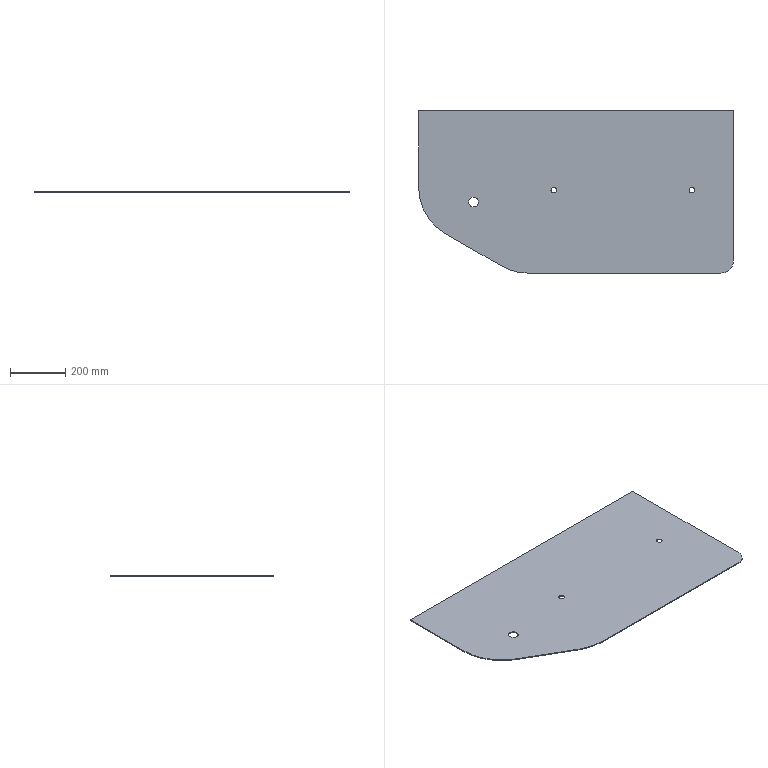Part | SolidWorks | features Extrusion 1 | 1 solid | 16 faces | box 1139 x 587 x 3 mm | volume 1890389 mm3 | cylinder 9 | plane 7 | commonest cylinder face diameters 20 x4 35 x2 390 x2 90 x1
STEP:
#1=CARTESIAN_POINT('',(-957.5,257.,3.));
#2=VERTEX_POINT('',#1);
#3=CARTESIAN_POINT('',(-922.5,257.,3.));
#4=VERTEX_POINT('',#3);
#5=CARTESIAN_POINT('',(-940.,257.,3.));
#6=DIRECTION('',(0.,0.,1.));
#7=DIRECTION('',(1.,0.,0.));
#8=AXIS2_PLACEMENT_3D('',#5,#6,#7);
#9=CIRCLE('',#8,17.5);
#10=EDGE_CURVE('',#2,#4,#9,.T.);
#11=ORIENTED_EDGE('',*,*,#10,.T.);
#12=CARTESIAN_POINT('',(-922.5,257.,0.));
#13=VERTEX_POINT('',#12);
#14=CARTESIAN_POINT('',(-922.5,257.,3.));
#15=DIRECTION('',(0.,0.,-1.));
#16=VECTOR('',#15,1000.);
#17=LINE('',#14,#16);
#18=EDGE_CURVE('',#4,#13,#17,.T.);
#19=ORIENTED_EDGE('',*,*,#18,.T.);
#20=CARTESIAN_POINT('',(-957.5,257.,0.));
#21=VERTEX_POINT('',#20);
#22=CARTESIAN_POINT('',(-940.,257.,0.));
#23=DIRECTION('',(0.,0.,1.));
#24=DIRECTION('',(1.,0.,0.));
#25=AXIS2_PLACEMENT_3D('',#22,#23,#24);
#26=CIRCLE('',#25,17.5);
#27=EDGE_CURVE('',#21,#13,#26,.T.);
#28=ORIENTED_EDGE('',*,*,#27,.F.);
#29=CARTESIAN_POINT('',(-957.5,257.,3.));
#30=DIRECTION('',(0.,0.,-1.));
#31=VECTOR('',#30,1000.);
#32=LINE('',#29,#31);
#33=EDGE_CURVE('',#2,#21,#32,.T.);
#34=ORIENTED_EDGE('',*,*,#33,.F.);
#35=EDGE_LOOP('',(#11,#19,#28,#34));
#36=FACE_OUTER_BOUND('',#35,.T.);
#37=CARTESIAN_POINT('',(-940.,257.,3.));
#38=DIRECTION('',(0.,0.,-1.));
#39=DIRECTION('',(-1.,0.,0.));
#40=AXIS2_PLACEMENT_3D('',#37,#38,#39);
#41=CYLINDRICAL_SURFACE('',#40,17.5);
#42=ADVANCED_FACE('',(#36),#41,.F.);
#43=CARTESIAN_POINT('',(-160.,300.,3.));
#44=VERTEX_POINT('',#43);
#45=CARTESIAN_POINT('',(-140.,300.,3.));
#46=VERTEX_POINT('',#45);
#47=CARTESIAN_POINT('',(-150.,300.,3.));
#48=DIRECTION('',(0.,0.,1.));
#49=DIRECTION('',(1.,0.,0.));
#50=AXIS2_PLACEMENT_3D('',#47,#48,#49);
#51=CIRCLE('',#50,10.);
#52=EDGE_CURVE('',#44,#46,#51,.T.);
#53=ORIENTED_EDGE('',*,*,#52,.T.);
#54=CARTESIAN_POINT('',(-140.,300.,0.));
#55=VERTEX_POINT('',#54);
#56=CARTESIAN_POINT('',(-140.,300.,3.));
#57=DIRECTION('',(0.,0.,-1.));
#58=VECTOR('',#57,1000.);
#59=LINE('',#56,#58);
#60=EDGE_CURVE('',#46,#55,#59,.T.);
#61=ORIENTED_EDGE('',*,*,#60,.T.);
#62=CARTESIAN_POINT('',(-160.,300.,0.));
#63=VERTEX_POINT('',#62);
#64=CARTESIAN_POINT('',(-150.,300.,0.));
#65=DIRECTION('',(0.,0.,1.));
#66=DIRECTION('',(1.,0.,0.));
#67=AXIS2_PLACEMENT_3D('',#64,#65,#66);
#68=CIRCLE('',#67,10.);
#69=EDGE_CURVE('',#63,#55,#68,.T.);
#70=ORIENTED_EDGE('',*,*,#69,.F.);
#71=CARTESIAN_POINT('',(-160.,300.,3.));
#72=DIRECTION('',(0.,0.,-1.));
#73=VECTOR('',#72,1000.);
#74=LINE('',#71,#73);
#75=EDGE_CURVE('',#44,#63,#74,.T.);
#76=ORIENTED_EDGE('',*,*,#75,.F.);
#77=EDGE_LOOP('',(#53,#61,#70,#76));
#78=FACE_OUTER_BOUND('',#77,.T.);
#79=CARTESIAN_POINT('',(-150.,300.,3.));
#80=DIRECTION('',(0.,0.,-1.));
#81=DIRECTION('',(-1.,0.,0.));
#82=AXIS2_PLACEMENT_3D('',#79,#80,#81);
#83=CYLINDRICAL_SURFACE('',#82,10.);
#84=ADVANCED_FACE('',(#78),#83,.F.);
#85=CARTESIAN_POINT('',(-660.,300.,3.));
#86=VERTEX_POINT('',#85);
#87=CARTESIAN_POINT('',(-640.,300.,3.));
#88=VERTEX_POINT('',#87);
#89=CARTESIAN_POINT('',(-650.,300.,3.));
#90=DIRECTION('',(0.,0.,1.));
#91=DIRECTION('',(1.,0.,0.));
#92=AXIS2_PLACEMENT_3D('',#89,#90,#91);
#93=CIRCLE('',#92,10.);
#94=EDGE_CURVE('',#86,#88,#93,.T.);
#95=ORIENTED_EDGE('',*,*,#94,.T.);
#96=CARTESIAN_POINT('',(-640.,300.,0.));
#97=VERTEX_POINT('',#96);
#98=CARTESIAN_POINT('',(-640.,300.,3.));
#99=DIRECTION('',(0.,0.,-1.));
#100=VECTOR('',#99,1000.);
#101=LINE('',#98,#100);
#102=EDGE_CURVE('',#88,#97,#101,.T.);
#103=ORIENTED_EDGE('',*,*,#102,.T.);
#104=CARTESIAN_POINT('',(-660.,300.,0.));
#105=VERTEX_POINT('',#104);
#106=CARTESIAN_POINT('',(-650.,300.,0.));
#107=DIRECTION('',(0.,0.,1.));
#108=DIRECTION('',(1.,0.,0.));
#109=AXIS2_PLACEMENT_3D('',#106,#107,#108);
#110=CIRCLE('',#109,10.);
#111=EDGE_CURVE('',#105,#97,#110,.T.);
#112=ORIENTED_EDGE('',*,*,#111,.F.);
#113=CARTESIAN_POINT('',(-660.,300.,3.));
#114=DIRECTION('',(0.,0.,-1.));
#115=VECTOR('',#114,1000.);
#116=LINE('',#113,#115);
#117=EDGE_CURVE('',#86,#105,#116,.T.);
#118=ORIENTED_EDGE('',*,*,#117,.F.);
#119=EDGE_LOOP('',(#95,#103,#112,#118));
#120=FACE_OUTER_BOUND('',#119,.T.);
#121=CARTESIAN_POINT('',(-650.,300.,3.));
#122=DIRECTION('',(0.,0.,-1.));
#123=DIRECTION('',(-1.,0.,0.));
#124=AXIS2_PLACEMENT_3D('',#121,#122,#123);
#125=CYLINDRICAL_SURFACE('',#124,10.);
#126=ADVANCED_FACE('',(#120),#125,.F.);
#127=ORIENTED_EDGE('',*,*,#52,.F.);
#128=CARTESIAN_POINT('',(-150.,300.,3.));
#129=DIRECTION('',(0.,0.,1.));
#130=DIRECTION('',(1.,0.,0.));
#131=AXIS2_PLACEMENT_3D('',#128,#129,#130);
#132=CIRCLE('',#131,10.);
#133=EDGE_CURVE('',#46,#44,#132,.T.);
#134=ORIENTED_EDGE('',*,*,#133,.F.);
#135=EDGE_LOOP('',(#127,#134));
#136=FACE_BOUND('',#135,.T.);
#137=CARTESIAN_POINT('',(0.,587.,3.));
#138=VERTEX_POINT('',#137);
#139=CARTESIAN_POINT('',(-1139.,587.,3.));
#140=VERTEX_POINT('',#139);
#141=CARTESIAN_POINT('',(0.,587.,3.));
#142=DIRECTION('',(-1.,0.,0.));
#143=VECTOR('',#142,1000.);
#144=LINE('',#141,#143);
#145=EDGE_CURVE('',#138,#140,#144,.T.);
#146=ORIENTED_EDGE('',*,*,#145,.T.);
#147=CARTESIAN_POINT('',(-1139.,311.192,3.));
#148=VERTEX_POINT('',#147);
#149=CARTESIAN_POINT('',(-1139.,587.,3.));
#150=DIRECTION('',(0.,-1.,0.));
#151=VECTOR('',#150,1000.);
#152=LINE('',#149,#151);
#153=EDGE_CURVE('',#140,#148,#152,.T.);
#154=ORIENTED_EDGE('',*,*,#153,.T.);
#155=CARTESIAN_POINT('',(-1041.5,142.317,3.));
#156=VERTEX_POINT('',#155);
#157=CARTESIAN_POINT('',(-944.,311.192,3.));
#158=DIRECTION('',(0.,0.,1.));
#159=DIRECTION('',(1.,0.,0.));
#160=AXIS2_PLACEMENT_3D('',#157,#158,#159);
#161=CIRCLE('',#160,195.);
#162=EDGE_CURVE('',#148,#156,#161,.T.);
#163=ORIENTED_EDGE('',*,*,#162,.T.);
#164=CARTESIAN_POINT('',(-840.25,26.125,3.));
#165=VERTEX_POINT('',#164);
#166=CARTESIAN_POINT('',(-840.25,26.125,3.));
#167=DIRECTION('',(0.866,-0.5,0.));
#168=VECTOR('',#167,1000.);
#169=LINE('',#166,#168);
#170=EDGE_CURVE('',#156,#165,#169,.T.);
#171=ORIENTED_EDGE('',*,*,#170,.T.);
#172=CARTESIAN_POINT('',(-742.75,0.,3.));
#173=VERTEX_POINT('',#172);
#174=CARTESIAN_POINT('',(-742.75,195.,3.));
#175=DIRECTION('',(0.,0.,1.));
#176=DIRECTION('',(-1.,0.,0.));
#177=AXIS2_PLACEMENT_3D('',#174,#175,#176);
#178=CIRCLE('',#177,195.);
#179=EDGE_CURVE('',#165,#173,#178,.T.);
#180=ORIENTED_EDGE('',*,*,#179,.T.);
#181=CARTESIAN_POINT('',(-45.,0.,3.));
#182=VERTEX_POINT('',#181);
#183=CARTESIAN_POINT('',(-45.,0.,3.));
#184=DIRECTION('',(1.,0.,0.));
#185=VECTOR('',#184,1000.);
#186=LINE('',#183,#185);
#187=EDGE_CURVE('',#173,#182,#186,.T.);
#188=ORIENTED_EDGE('',*,*,#187,.T.);
#189=CARTESIAN_POINT('',(0.,45.,3.));
#190=VERTEX_POINT('',#189);
#191=CARTESIAN_POINT('',(-45.,45.,3.));
#192=DIRECTION('',(0.,0.,1.));
#193=DIRECTION('',(-1.,0.,0.));
#194=AXIS2_PLACEMENT_3D('',#191,#192,#193);
#195=CIRCLE('',#194,45.);
#196=EDGE_CURVE('',#182,#190,#195,.T.);
#197=ORIENTED_EDGE('',*,*,#196,.T.);
#198=CARTESIAN_POINT('',(0.,587.,3.));
#199=DIRECTION('',(0.,1.,0.));
#200=VECTOR('',#199,1000.);
#201=LINE('',#198,#200);
#202=EDGE_CURVE('',#190,#138,#201,.T.);
#203=ORIENTED_EDGE('',*,*,#202,.T.);
#204=EDGE_LOOP('',(#146,#154,#163,#171,#180,#188,#197,#203));
#205=FACE_OUTER_BOUND('',#204,.T.);
#206=ORIENTED_EDGE('',*,*,#94,.F.);
#207=CARTESIAN_POINT('',(-650.,300.,3.));
#208=DIRECTION('',(0.,0.,1.));
#209=DIRECTION('',(1.,0.,0.));
#210=AXIS2_PLACEMENT_3D('',#207,#208,#209);
#211=CIRCLE('',#210,10.);
#212=EDGE_CURVE('',#88,#86,#211,.T.);
#213=ORIENTED_EDGE('',*,*,#212,.F.);
#214=EDGE_LOOP('',(#206,#213));
#215=FACE_BOUND('',#214,.T.);
#216=ORIENTED_EDGE('',*,*,#10,.F.);
#217=CARTESIAN_POINT('',(-940.,257.,3.));
#218=DIRECTION('',(0.,0.,1.));
#219=DIRECTION('',(1.,0.,0.));
#220=AXIS2_PLACEMENT_3D('',#217,#218,#219);
#221=CIRCLE('',#220,17.5);
#222=EDGE_CURVE('',#4,#2,#221,.T.);
#223=ORIENTED_EDGE('',*,*,#222,.F.);
#224=EDGE_LOOP('',(#216,#223));
#225=FACE_BOUND('',#224,.T.);
#226=CARTESIAN_POINT('',(-944.,311.192,3.));
#227=DIRECTION('',(0.,0.,1.));
#228=DIRECTION('',(1.,0.,0.));
#229=AXIS2_PLACEMENT_3D('',#226,#227,#228);
#230=PLANE('',#229);
#231=ADVANCED_FACE('',(#136,#205,#215,#225),#230,.T.);
#232=ORIENTED_EDGE('',*,*,#69,.T.);
#233=CARTESIAN_POINT('',(-150.,300.,0.));
#234=DIRECTION('',(0.,0.,1.));
#235=DIRECTION('',(1.,0.,0.));
#236=AXIS2_PLACEMENT_3D('',#233,#234,#235);
#237=CIRCLE('',#236,10.);
#238=EDGE_CURVE('',#55,#63,#237,.T.);
#239=ORIENTED_EDGE('',*,*,#238,.T.);
#240=EDGE_LOOP('',(#232,#239));
#241=FACE_BOUND('',#240,.T.);
#242=CARTESIAN_POINT('',(0.,587.,0.));
#243=VERTEX_POINT('',#242);
#244=CARTESIAN_POINT('',(-1139.,587.,0.));
#245=VERTEX_POINT('',#244);
#246=CARTESIAN_POINT('',(0.,587.,0.));
#247=DIRECTION('',(-1.,0.,0.));
#248=VECTOR('',#247,1000.);
#249=LINE('',#246,#248);
#250=EDGE_CURVE('',#243,#245,#249,.T.);
#251=ORIENTED_EDGE('',*,*,#250,.F.);
#252=CARTESIAN_POINT('',(0.,45.,0.));
#253=VERTEX_POINT('',#252);
#254=CARTESIAN_POINT('',(0.,587.,0.));
#255=DIRECTION('',(0.,1.,0.));
#256=VECTOR('',#255,1000.);
#257=LINE('',#254,#256);
#258=EDGE_CURVE('',#253,#243,#257,.T.);
#259=ORIENTED_EDGE('',*,*,#258,.F.);
#260=CARTESIAN_POINT('',(-45.,0.,0.));
#261=VERTEX_POINT('',#260);
#262=CARTESIAN_POINT('',(-45.,45.,0.));
#263=DIRECTION('',(0.,0.,1.));
#264=DIRECTION('',(-1.,0.,0.));
#265=AXIS2_PLACEMENT_3D('',#262,#263,#264);
#266=CIRCLE('',#265,45.);
#267=EDGE_CURVE('',#261,#253,#266,.T.);
#268=ORIENTED_EDGE('',*,*,#267,.F.);
#269=CARTESIAN_POINT('',(-742.75,0.,0.));
#270=VERTEX_POINT('',#269);
#271=CARTESIAN_POINT('',(-45.,0.,0.));
#272=DIRECTION('',(1.,0.,0.));
#273=VECTOR('',#272,1000.);
#274=LINE('',#271,#273);
#275=EDGE_CURVE('',#270,#261,#274,.T.);
#276=ORIENTED_EDGE('',*,*,#275,.F.);
#277=CARTESIAN_POINT('',(-840.25,26.125,0.));
#278=VERTEX_POINT('',#277);
#279=CARTESIAN_POINT('',(-742.75,195.,0.));
#280=DIRECTION('',(0.,0.,1.));
#281=DIRECTION('',(-1.,0.,0.));
#282=AXIS2_PLACEMENT_3D('',#279,#280,#281);
#283=CIRCLE('',#282,195.);
#284=EDGE_CURVE('',#278,#270,#283,.T.);
#285=ORIENTED_EDGE('',*,*,#284,.F.);
#286=CARTESIAN_POINT('',(-1041.5,142.317,0.));
#287=VERTEX_POINT('',#286);
#288=CARTESIAN_POINT('',(-840.25,26.125,0.));
#289=DIRECTION('',(0.866,-0.5,0.));
#290=VECTOR('',#289,1000.);
#291=LINE('',#288,#290);
#292=EDGE_CURVE('',#287,#278,#291,.T.);
#293=ORIENTED_EDGE('',*,*,#292,.F.);
#294=CARTESIAN_POINT('',(-1139.,311.192,0.));
#295=VERTEX_POINT('',#294);
#296=CARTESIAN_POINT('',(-944.,311.192,0.));
#297=DIRECTION('',(0.,0.,1.));
#298=DIRECTION('',(1.,0.,0.));
#299=AXIS2_PLACEMENT_3D('',#296,#297,#298);
#300=CIRCLE('',#299,195.);
#301=EDGE_CURVE('',#295,#287,#300,.T.);
#302=ORIENTED_EDGE('',*,*,#301,.F.);
#303=CARTESIAN_POINT('',(-1139.,587.,0.));
#304=DIRECTION('',(0.,-1.,0.));
#305=VECTOR('',#304,1000.);
#306=LINE('',#303,#305);
#307=EDGE_CURVE('',#245,#295,#306,.T.);
#308=ORIENTED_EDGE('',*,*,#307,.F.);
#309=EDGE_LOOP('',(#251,#259,#268,#276,#285,#293,#302,#308));
#310=FACE_OUTER_BOUND('',#309,.T.);
#311=ORIENTED_EDGE('',*,*,#111,.T.);
#312=CARTESIAN_POINT('',(-650.,300.,0.));
#313=DIRECTION('',(0.,0.,1.));
#314=DIRECTION('',(1.,0.,0.));
#315=AXIS2_PLACEMENT_3D('',#312,#313,#314);
#316=CIRCLE('',#315,10.);
#317=EDGE_CURVE('',#97,#105,#316,.T.);
#318=ORIENTED_EDGE('',*,*,#317,.T.);
#319=EDGE_LOOP('',(#311,#318));
#320=FACE_BOUND('',#319,.T.);
#321=ORIENTED_EDGE('',*,*,#27,.T.);
#322=CARTESIAN_POINT('',(-940.,257.,0.));
#323=DIRECTION('',(0.,0.,1.));
#324=DIRECTION('',(1.,0.,0.));
#325=AXIS2_PLACEMENT_3D('',#322,#323,#324);
#326=CIRCLE('',#325,17.5);
#327=EDGE_CURVE('',#13,#21,#326,.T.);
#328=ORIENTED_EDGE('',*,*,#327,.T.);
#329=EDGE_LOOP('',(#321,#328));
#330=FACE_BOUND('',#329,.T.);
#331=CARTESIAN_POINT('',(-944.,311.192,0.));
#332=DIRECTION('',(0.,0.,1.));
#333=DIRECTION('',(1.,0.,0.));
#334=AXIS2_PLACEMENT_3D('',#331,#332,#333);
#335=PLANE('',#334);
#336=ADVANCED_FACE('',(#241,#310,#320,#330),#335,.F.);
#337=ORIENTED_EDGE('',*,*,#250,.T.);
#338=CARTESIAN_POINT('',(-1139.,587.,3.));
#339=DIRECTION('',(0.,0.,-1.));
#340=VECTOR('',#339,1000.);
#341=LINE('',#338,#340);
#342=EDGE_CURVE('',#140,#245,#341,.T.);
#343=ORIENTED_EDGE('',*,*,#342,.F.);
#344=ORIENTED_EDGE('',*,*,#145,.F.);
#345=CARTESIAN_POINT('',(0.,587.,3.));
#346=DIRECTION('',(0.,0.,-1.));
#347=VECTOR('',#346,1000.);
#348=LINE('',#345,#347);
#349=EDGE_CURVE('',#138,#243,#348,.T.);
#350=ORIENTED_EDGE('',*,*,#349,.T.);
#351=EDGE_LOOP('',(#337,#343,#344,#350));
#352=FACE_OUTER_BOUND('',#351,.T.);
#353=CARTESIAN_POINT('',(0.,587.,3.));
#354=DIRECTION('',(0.,-1.,0.));
#355=DIRECTION('',(1.,0.,0.));
#356=AXIS2_PLACEMENT_3D('',#353,#354,#355);
#357=PLANE('',#356);
#358=ADVANCED_FACE('',(#352),#357,.F.);
#359=ORIENTED_EDGE('',*,*,#307,.T.);
#360=CARTESIAN_POINT('',(-1139.,311.192,3.));
#361=DIRECTION('',(0.,0.,-1.));
#362=VECTOR('',#361,1000.);
#363=LINE('',#360,#362);
#364=EDGE_CURVE('',#148,#295,#363,.T.);
#365=ORIENTED_EDGE('',*,*,#364,.F.);
#366=ORIENTED_EDGE('',*,*,#153,.F.);
#367=ORIENTED_EDGE('',*,*,#342,.T.);
#368=EDGE_LOOP('',(#359,#365,#366,#367));
#369=FACE_OUTER_BOUND('',#368,.T.);
#370=CARTESIAN_POINT('',(-1139.,587.,3.));
#371=DIRECTION('',(1.,0.,0.));
#372=DIRECTION('',(0.,1.,0.));
#373=AXIS2_PLACEMENT_3D('',#370,#371,#372);
#374=PLANE('',#373);
#375=ADVANCED_FACE('',(#369),#374,.F.);
#376=ORIENTED_EDGE('',*,*,#301,.T.);
#377=CARTESIAN_POINT('',(-1041.5,142.317,3.));
#378=DIRECTION('',(0.,0.,-1.));
#379=VECTOR('',#378,1000.);
#380=LINE('',#377,#379);
#381=EDGE_CURVE('',#156,#287,#380,.T.);
#382=ORIENTED_EDGE('',*,*,#381,.F.);
#383=ORIENTED_EDGE('',*,*,#162,.F.);
#384=ORIENTED_EDGE('',*,*,#364,.T.);
#385=EDGE_LOOP('',(#376,#382,#383,#384));
#386=FACE_OUTER_BOUND('',#385,.T.);
#387=CARTESIAN_POINT('',(-944.,311.192,3.));
#388=DIRECTION('',(0.,0.,-1.));
#389=DIRECTION('',(-1.,0.,0.));
#390=AXIS2_PLACEMENT_3D('',#387,#388,#389);
#391=CYLINDRICAL_SURFACE('',#390,195.);
#392=ADVANCED_FACE('',(#386),#391,.T.);
#393=ORIENTED_EDGE('',*,*,#292,.T.);
#394=CARTESIAN_POINT('',(-840.25,26.125,3.));
#395=DIRECTION('',(0.,0.,-1.));
#396=VECTOR('',#395,1000.);
#397=LINE('',#394,#396);
#398=EDGE_CURVE('',#165,#278,#397,.T.);
#399=ORIENTED_EDGE('',*,*,#398,.F.);
#400=ORIENTED_EDGE('',*,*,#170,.F.);
#401=ORIENTED_EDGE('',*,*,#381,.T.);
#402=EDGE_LOOP('',(#393,#399,#400,#401));
#403=FACE_OUTER_BOUND('',#402,.T.);
#404=CARTESIAN_POINT('',(-840.25,26.125,3.));
#405=DIRECTION('',(0.5,0.866,0.));
#406=DIRECTION('',(-0.866,0.5,0.));
#407=AXIS2_PLACEMENT_3D('',#404,#405,#406);
#408=PLANE('',#407);
#409=ADVANCED_FACE('',(#403),#408,.F.);
#410=ORIENTED_EDGE('',*,*,#284,.T.);
#411=CARTESIAN_POINT('',(-742.75,0.,3.));
#412=DIRECTION('',(0.,0.,-1.));
#413=VECTOR('',#412,1000.);
#414=LINE('',#411,#413);
#415=EDGE_CURVE('',#173,#270,#414,.T.);
#416=ORIENTED_EDGE('',*,*,#415,.F.);
#417=ORIENTED_EDGE('',*,*,#179,.F.);
#418=ORIENTED_EDGE('',*,*,#398,.T.);
#419=EDGE_LOOP('',(#410,#416,#417,#418));
#420=FACE_OUTER_BOUND('',#419,.T.);
#421=CARTESIAN_POINT('',(-742.75,195.,3.));
#422=DIRECTION('',(0.,0.,-1.));
#423=DIRECTION('',(-1.,0.,0.));
#424=AXIS2_PLACEMENT_3D('',#421,#422,#423);
#425=CYLINDRICAL_SURFACE('',#424,195.);
#426=ADVANCED_FACE('',(#420),#425,.T.);
#427=ORIENTED_EDGE('',*,*,#275,.T.);
#428=CARTESIAN_POINT('',(-45.,0.,3.));
#429=DIRECTION('',(0.,0.,-1.));
#430=VECTOR('',#429,1000.);
#431=LINE('',#428,#430);
#432=EDGE_CURVE('',#182,#261,#431,.T.);
#433=ORIENTED_EDGE('',*,*,#432,.F.);
#434=ORIENTED_EDGE('',*,*,#187,.F.);
#435=ORIENTED_EDGE('',*,*,#415,.T.);
#436=EDGE_LOOP('',(#427,#433,#434,#435));
#437=FACE_OUTER_BOUND('',#436,.T.);
#438=CARTESIAN_POINT('',(-45.,0.,3.));
#439=DIRECTION('',(0.,1.,0.));
#440=DIRECTION('',(-1.,0.,0.));
#441=AXIS2_PLACEMENT_3D('',#438,#439,#440);
#442=PLANE('',#441);
#443=ADVANCED_FACE('',(#437),#442,.F.);
#444=ORIENTED_EDGE('',*,*,#267,.T.);
#445=CARTESIAN_POINT('',(0.,45.,3.));
#446=DIRECTION('',(0.,0.,-1.));
#447=VECTOR('',#446,1000.);
#448=LINE('',#445,#447);
#449=EDGE_CURVE('',#190,#253,#448,.T.);
#450=ORIENTED_EDGE('',*,*,#449,.F.);
#451=ORIENTED_EDGE('',*,*,#196,.F.);
#452=ORIENTED_EDGE('',*,*,#432,.T.);
#453=EDGE_LOOP('',(#444,#450,#451,#452));
#454=FACE_OUTER_BOUND('',#453,.T.);
#455=CARTESIAN_POINT('',(-45.,45.,3.));
#456=DIRECTION('',(0.,0.,-1.));
#457=DIRECTION('',(-1.,0.,0.));
#458=AXIS2_PLACEMENT_3D('',#455,#456,#457);
#459=CYLINDRICAL_SURFACE('',#458,45.);
#460=ADVANCED_FACE('',(#454),#459,.T.);
#461=ORIENTED_EDGE('',*,*,#258,.T.);
#462=ORIENTED_EDGE('',*,*,#349,.F.);
#463=ORIENTED_EDGE('',*,*,#202,.F.);
#464=ORIENTED_EDGE('',*,*,#449,.T.);
#465=EDGE_LOOP('',(#461,#462,#463,#464));
#466=FACE_OUTER_BOUND('',#465,.T.);
#467=CARTESIAN_POINT('',(0.,587.,3.));
#468=DIRECTION('',(-1.,0.,0.));
#469=DIRECTION('',(0.,0.,1.));
#470=AXIS2_PLACEMENT_3D('',#467,#468,#469);
#471=PLANE('',#470);
#472=ADVANCED_FACE('',(#466),#471,.F.);
#473=ORIENTED_EDGE('',*,*,#102,.F.);
#474=ORIENTED_EDGE('',*,*,#212,.T.);
#475=ORIENTED_EDGE('',*,*,#117,.T.);
#476=ORIENTED_EDGE('',*,*,#317,.F.);
#477=EDGE_LOOP('',(#473,#474,#475,#476));
#478=FACE_OUTER_BOUND('',#477,.T.);
#479=CARTESIAN_POINT('',(-650.,300.,3.));
#480=DIRECTION('',(0.,0.,-1.));
#481=DIRECTION('',(-1.,0.,0.));
#482=AXIS2_PLACEMENT_3D('',#479,#480,#481);
#483=CYLINDRICAL_SURFACE('',#482,10.);
#484=ADVANCED_FACE('',(#478),#483,.F.);
#485=ORIENTED_EDGE('',*,*,#60,.F.);
#486=ORIENTED_EDGE('',*,*,#133,.T.);
#487=ORIENTED_EDGE('',*,*,#75,.T.);
#488=ORIENTED_EDGE('',*,*,#238,.F.);
#489=EDGE_LOOP('',(#485,#486,#487,#488));
#490=FACE_OUTER_BOUND('',#489,.T.);
#491=CARTESIAN_POINT('',(-150.,300.,3.));
#492=DIRECTION('',(0.,0.,-1.));
#493=DIRECTION('',(-1.,0.,0.));
#494=AXIS2_PLACEMENT_3D('',#491,#492,#493);
#495=CYLINDRICAL_SURFACE('',#494,10.);
#496=ADVANCED_FACE('',(#490),#495,.F.);
#497=ORIENTED_EDGE('',*,*,#18,.F.);
#498=ORIENTED_EDGE('',*,*,#222,.T.);
#499=ORIENTED_EDGE('',*,*,#33,.T.);
#500=ORIENTED_EDGE('',*,*,#327,.F.);
#501=EDGE_LOOP('',(#497,#498,#499,#500));
#502=FACE_OUTER_BOUND('',#501,.T.);
#503=CARTESIAN_POINT('',(-940.,257.,3.));
#504=DIRECTION('',(0.,0.,-1.));
#505=DIRECTION('',(-1.,0.,0.));
#506=AXIS2_PLACEMENT_3D('',#503,#504,#505);
#507=CYLINDRICAL_SURFACE('',#506,17.5);
#508=ADVANCED_FACE('',(#502),#507,.F.);
#509=CLOSED_SHELL('',(#42,#84,#126,#231,#336,#358,#375,#392,#409,#426,#443,#460,#472,#484,#496,#508));
#510=MANIFOLD_SOLID_BREP('',#509);
#511=CARTESIAN_POINT('',(0.,0.,0.));
#512=DIRECTION('',(0.,0.,1.));
#513=DIRECTION('',(1.,0.,0.));
#514=AXIS2_PLACEMENT_3D('',#511,#512,#513);
#515=(LENGTH_UNIT()NAMED_UNIT(*)SI_UNIT(.MILLI.,.METRE.));
#516=UNCERTAINTY_MEASURE_WITH_UNIT(LENGTH_MEASURE(0.00001),#515,'','');
#517=(NAMED_UNIT(*)PLANE_ANGLE_UNIT()SI_UNIT($,.RADIAN.));
#518=(NAMED_UNIT(*)SI_UNIT($,.STERADIAN.)SOLID_ANGLE_UNIT());
#519=(GEOMETRIC_REPRESENTATION_CONTEXT(3)GLOBAL_UNCERTAINTY_ASSIGNED_CONTEXT((#516))GLOBAL_UNIT_ASSIGNED_CONTEXT((#515,#517,#518))REPRESENTATION_CONTEXT('',''));
#520=ADVANCED_BREP_SHAPE_REPRESENTATION('',(#510,#514),#519);